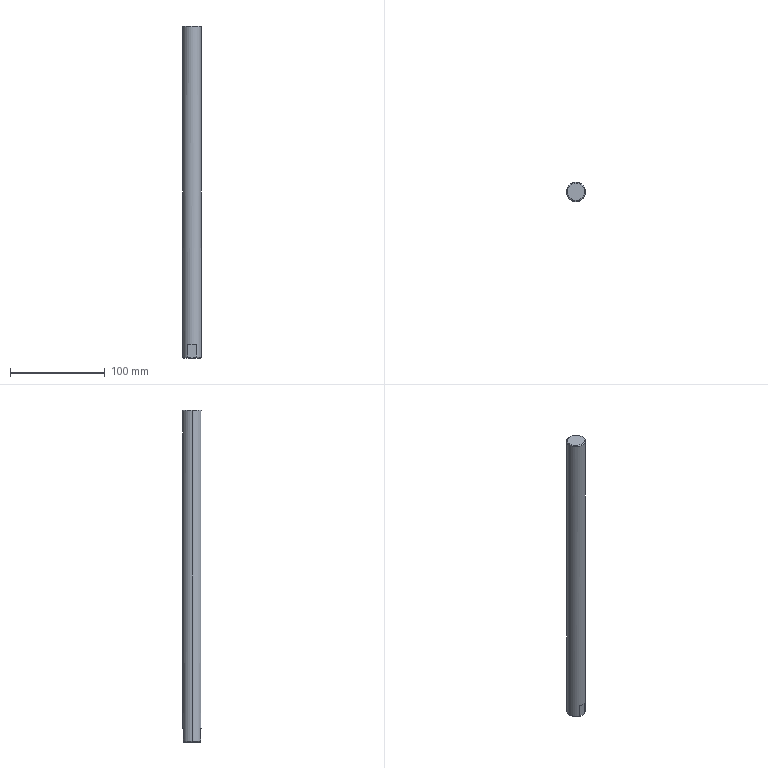Part | STEP file | KF-2212-050-003 | 1 solid | 17 faces | box 20 x 20 x 350 mm | volume 109026 mm3 | plane 6 | torus 5 | cylinder 4 | cone 2 | commonest cylinder face diameters 6.8 x2 20 x2
STEP:
#1=CARTESIAN_POINT('',(3.4,0.,19.75));
#2=VERTEX_POINT('',#1);
#3=CARTESIAN_POINT('',(-3.4,0.,19.75));
#4=VERTEX_POINT('',#3);
#5=CARTESIAN_POINT('',(0.,0.,19.75));
#6=DIRECTION('',(0.,0.,-1.));
#7=DIRECTION('',(-1.,0.,0.));
#8=AXIS2_PLACEMENT_3D('',#5,#6,#7);
#9=CIRCLE('',#8,3.4);
#10=EDGE_CURVE('',#2,#4,#9,.T.);
#11=ORIENTED_EDGE('',*,*,#10,.F.);
#12=CARTESIAN_POINT('',(3.4,0.,0.));
#13=VERTEX_POINT('',#12);
#14=CARTESIAN_POINT('',(3.4,0.,0.));
#15=DIRECTION('',(0.,0.,-1.));
#16=VECTOR('',#15,1000.);
#17=LINE('',#14,#16);
#18=EDGE_CURVE('',#2,#13,#17,.T.);
#19=ORIENTED_EDGE('',*,*,#18,.T.);
#20=CARTESIAN_POINT('',(-3.4,0.,0.));
#21=VERTEX_POINT('',#20);
#22=CARTESIAN_POINT('',(0.,0.,0.));
#23=DIRECTION('',(0.,0.,-1.));
#24=DIRECTION('',(-1.,0.,0.));
#25=AXIS2_PLACEMENT_3D('',#22,#23,#24);
#26=CIRCLE('',#25,3.4);
#27=EDGE_CURVE('',#13,#21,#26,.T.);
#28=ORIENTED_EDGE('',*,*,#27,.T.);
#29=CARTESIAN_POINT('',(-3.4,0.,0.));
#30=DIRECTION('',(0.,0.,-1.));
#31=VECTOR('',#30,1000.);
#32=LINE('',#29,#31);
#33=EDGE_CURVE('',#4,#21,#32,.T.);
#34=ORIENTED_EDGE('',*,*,#33,.F.);
#35=EDGE_LOOP('',(#11,#19,#28,#34));
#36=FACE_OUTER_BOUND('',#35,.T.);
#37=CARTESIAN_POINT('',(0.,0.,0.));
#38=DIRECTION('',(0.,0.,-1.));
#39=DIRECTION('',(-1.,0.,0.));
#40=AXIS2_PLACEMENT_3D('',#37,#38,#39);
#41=CYLINDRICAL_SURFACE('',#40,3.4);
#42=ADVANCED_FACE('',(#36),#41,.F.);
#43=CARTESIAN_POINT('',(0.,0.,21.793));
#44=VERTEX_POINT('',#43);
#45=CARTESIAN_POINT('',(-3.4,0.,19.75));
#46=DIRECTION('',(-0.8572,0.,-0.515));
#47=VECTOR('',#46,1000.);
#48=LINE('',#45,#47);
#49=EDGE_CURVE('',#44,#4,#48,.T.);
#50=ORIENTED_EDGE('',*,*,#49,.F.);
#51=CARTESIAN_POINT('',(3.4,0.,19.75));
#52=DIRECTION('',(0.8572,0.,-0.515));
#53=VECTOR('',#52,1000.);
#54=LINE('',#51,#53);
#55=EDGE_CURVE('',#44,#2,#54,.T.);
#56=ORIENTED_EDGE('',*,*,#55,.T.);
#57=ORIENTED_EDGE('',*,*,#10,.T.);
#58=EDGE_LOOP('',(#50,#56,#57));
#59=FACE_OUTER_BOUND('',#58,.T.);
#60=CARTESIAN_POINT('',(0.,0.,19.75));
#61=DIRECTION('',(0.,0.,-1.));
#62=DIRECTION('',(-1.,0.,0.));
#63=AXIS2_PLACEMENT_3D('',#60,#61,#62);
#64=CONICAL_SURFACE('',#63,3.4,1.03);
#65=ADVANCED_FACE('',(#59),#64,.F.);
#66=CARTESIAN_POINT('',(9.,0.,0.));
#67=VERTEX_POINT('',#66);
#68=CARTESIAN_POINT('',(0.,-9.,0.));
#69=VERTEX_POINT('',#68);
#70=CARTESIAN_POINT('',(0.,0.,0.));
#71=DIRECTION('',(0.,0.,-1.));
#72=DIRECTION('',(1.,0.,0.));
#73=AXIS2_PLACEMENT_3D('',#70,#71,#72);
#74=CIRCLE('',#73,9.);
#75=EDGE_CURVE('',#67,#69,#74,.T.);
#76=ORIENTED_EDGE('',*,*,#75,.F.);
#77=CARTESIAN_POINT('',(10.,0.,1.));
#78=VERTEX_POINT('',#77);
#79=CARTESIAN_POINT('',(9.,0.,1.));
#80=DIRECTION('',(0.,-1.,0.));
#81=DIRECTION('',(0.,0.,-1.));
#82=AXIS2_PLACEMENT_3D('',#79,#80,#81);
#83=CIRCLE('',#82,1.);
#84=EDGE_CURVE('',#67,#78,#83,.T.);
#85=ORIENTED_EDGE('',*,*,#84,.T.);
#86=CARTESIAN_POINT('',(4.359,-9.,1.));
#87=VERTEX_POINT('',#86);
#88=CARTESIAN_POINT('',(0.,0.,1.));
#89=DIRECTION('',(0.,0.,1.));
#90=DIRECTION('',(1.,0.,0.));
#91=AXIS2_PLACEMENT_3D('',#88,#89,#90);
#92=CIRCLE('',#91,10.);
#93=EDGE_CURVE('',#87,#78,#92,.T.);
#94=ORIENTED_EDGE('',*,*,#93,.F.);
#95=CARTESIAN_POINT('',(0.,-9.,0.));
#96=CARTESIAN_POINT('',(0.3943,-9.,0.));
#97=CARTESIAN_POINT('',(0.7886,-9.,-0.0009886));
#98=CARTESIAN_POINT('',(1.577,-9.,0.006989));
#99=CARTESIAN_POINT('',(1.972,-9.,0.01581));
#100=CARTESIAN_POINT('',(2.561,-9.,0.06379));
#101=CARTESIAN_POINT('',(2.756,-9.,0.0857));
#102=CARTESIAN_POINT('',(3.144,-9.,0.1503));
#103=CARTESIAN_POINT('',(3.339,-9.,0.1931));
#104=CARTESIAN_POINT('',(3.62,-9.,0.2846));
#105=CARTESIAN_POINT('',(3.712,-9.,0.3197));
#106=CARTESIAN_POINT('',(3.89,-9.,0.4033));
#107=CARTESIAN_POINT('',(3.977,-9.,0.4522));
#108=CARTESIAN_POINT('',(4.137,-9.,0.5697));
#109=CARTESIAN_POINT('',(4.211,-9.,0.6387));
#110=CARTESIAN_POINT('',(4.322,-9.,0.8026));
#111=CARTESIAN_POINT('',(4.359,-9.,0.9011));
#112=CARTESIAN_POINT('',(4.359,-9.,1.));
#113=B_SPLINE_CURVE_WITH_KNOTS('',3,(#95,#96,#97,#98,#99,#100,#101,#102,#103,#104,#105,#106,#107,#108,#109,#110,#111,#112),.UNSPECIFIED.,.F.,.F.,(4,2,2,2,2,2,2,2,4),(0.,0.001183,0.002366,0.002957,0.003549,0.003844,0.00414,0.004436,0.004731),.UNSPECIFIED.);
#114=EDGE_CURVE('',#69,#87,#113,.T.);
#115=ORIENTED_EDGE('',*,*,#114,.F.);
#116=EDGE_LOOP('',(#76,#85,#94,#115));
#117=FACE_OUTER_BOUND('',#116,.T.);
#118=CARTESIAN_POINT('',(0.,0.,1.));
#119=DIRECTION('',(0.,0.,1.));
#120=DIRECTION('',(1.,0.,0.));
#121=AXIS2_PLACEMENT_3D('',#118,#119,#120);
#122=TOROIDAL_SURFACE('',#121,9.,1.);
#123=ADVANCED_FACE('',(#117),#122,.T.);
#124=CARTESIAN_POINT('',(-10.,0.,349.));
#125=VERTEX_POINT('',#124);
#126=CARTESIAN_POINT('',(10.,0.,349.));
#127=VERTEX_POINT('',#126);
#128=CARTESIAN_POINT('',(0.,0.,349.));
#129=DIRECTION('',(0.,0.,-1.));
#130=DIRECTION('',(1.,0.,0.));
#131=AXIS2_PLACEMENT_3D('',#128,#129,#130);
#132=CIRCLE('',#131,10.);
#133=EDGE_CURVE('',#125,#127,#132,.T.);
#134=ORIENTED_EDGE('',*,*,#133,.F.);
#135=CARTESIAN_POINT('',(-9.,0.,350.));
#136=VERTEX_POINT('',#135);
#137=CARTESIAN_POINT('',(-9.,0.,349.));
#138=DIRECTION('',(0.,1.,0.));
#139=DIRECTION('',(-1.,0.,0.));
#140=AXIS2_PLACEMENT_3D('',#137,#138,#139);
#141=CIRCLE('',#140,1.);
#142=EDGE_CURVE('',#125,#136,#141,.T.);
#143=ORIENTED_EDGE('',*,*,#142,.T.);
#144=CARTESIAN_POINT('',(9.,0.,350.));
#145=VERTEX_POINT('',#144);
#146=CARTESIAN_POINT('',(0.,0.,350.));
#147=DIRECTION('',(0.,0.,1.));
#148=DIRECTION('',(1.,0.,0.));
#149=AXIS2_PLACEMENT_3D('',#146,#147,#148);
#150=CIRCLE('',#149,9.);
#151=EDGE_CURVE('',#145,#136,#150,.T.);
#152=ORIENTED_EDGE('',*,*,#151,.F.);
#153=CARTESIAN_POINT('',(9.,0.,349.));
#154=DIRECTION('',(0.,-1.,0.));
#155=DIRECTION('',(0.,0.,-1.));
#156=AXIS2_PLACEMENT_3D('',#153,#154,#155);
#157=CIRCLE('',#156,1.);
#158=EDGE_CURVE('',#127,#145,#157,.T.);
#159=ORIENTED_EDGE('',*,*,#158,.F.);
#160=EDGE_LOOP('',(#134,#143,#152,#159));
#161=FACE_OUTER_BOUND('',#160,.T.);
#162=CARTESIAN_POINT('',(0.,0.,349.));
#163=DIRECTION('',(0.,0.,1.));
#164=DIRECTION('',(1.,0.,0.));
#165=AXIS2_PLACEMENT_3D('',#162,#163,#164);
#166=TOROIDAL_SURFACE('',#165,9.,1.);
#167=ADVANCED_FACE('',(#161),#166,.T.);
#168=ORIENTED_EDGE('',*,*,#133,.T.);
#169=CARTESIAN_POINT('',(10.,0.,350.));
#170=DIRECTION('',(0.,0.,-1.));
#171=VECTOR('',#170,1000.);
#172=LINE('',#169,#171);
#173=EDGE_CURVE('',#127,#78,#172,.T.);
#174=ORIENTED_EDGE('',*,*,#173,.T.);
#175=CARTESIAN_POINT('',(4.359,9.,1.));
#176=VERTEX_POINT('',#175);
#177=CARTESIAN_POINT('',(0.,0.,1.));
#178=DIRECTION('',(0.,0.,1.));
#179=DIRECTION('',(1.,0.,0.));
#180=AXIS2_PLACEMENT_3D('',#177,#178,#179);
#181=CIRCLE('',#180,10.);
#182=EDGE_CURVE('',#78,#176,#181,.T.);
#183=ORIENTED_EDGE('',*,*,#182,.T.);
#184=CARTESIAN_POINT('',(4.359,9.,14.));
#185=VERTEX_POINT('',#184);
#186=CARTESIAN_POINT('',(4.359,9.,350.));
#187=DIRECTION('',(0.,0.,1.));
#188=VECTOR('',#187,1000.);
#189=LINE('',#186,#188);
#190=EDGE_CURVE('',#176,#185,#189,.T.);
#191=ORIENTED_EDGE('',*,*,#190,.T.);
#192=CARTESIAN_POINT('',(-4.359,9.,14.));
#193=VERTEX_POINT('',#192);
#194=CARTESIAN_POINT('',(0.,0.,14.));
#195=DIRECTION('',(0.,0.,-1.));
#196=DIRECTION('',(-1.,0.,0.));
#197=AXIS2_PLACEMENT_3D('',#194,#195,#196);
#198=CIRCLE('',#197,10.);
#199=EDGE_CURVE('',#193,#185,#198,.T.);
#200=ORIENTED_EDGE('',*,*,#199,.F.);
#201=CARTESIAN_POINT('',(-4.359,9.,1.));
#202=VERTEX_POINT('',#201);
#203=CARTESIAN_POINT('',(-4.359,9.,350.));
#204=DIRECTION('',(0.,0.,-1.));
#205=VECTOR('',#204,1000.);
#206=LINE('',#203,#205);
#207=EDGE_CURVE('',#193,#202,#206,.T.);
#208=ORIENTED_EDGE('',*,*,#207,.T.);
#209=CARTESIAN_POINT('',(-10.,0.,1.));
#210=VERTEX_POINT('',#209);
#211=CARTESIAN_POINT('',(0.,0.,1.));
#212=DIRECTION('',(0.,0.,1.));
#213=DIRECTION('',(1.,0.,0.));
#214=AXIS2_PLACEMENT_3D('',#211,#212,#213);
#215=CIRCLE('',#214,10.);
#216=EDGE_CURVE('',#202,#210,#215,.T.);
#217=ORIENTED_EDGE('',*,*,#216,.T.);
#218=CARTESIAN_POINT('',(-10.,0.,350.));
#219=DIRECTION('',(0.,0.,-1.));
#220=VECTOR('',#219,1000.);
#221=LINE('',#218,#220);
#222=EDGE_CURVE('',#125,#210,#221,.T.);
#223=ORIENTED_EDGE('',*,*,#222,.F.);
#224=EDGE_LOOP('',(#168,#174,#183,#191,#200,#208,#217,#223));
#225=FACE_OUTER_BOUND('',#224,.T.);
#226=CARTESIAN_POINT('',(0.,0.,350.));
#227=DIRECTION('',(0.,0.,-1.));
#228=DIRECTION('',(-1.,0.,0.));
#229=AXIS2_PLACEMENT_3D('',#226,#227,#228);
#230=CYLINDRICAL_SURFACE('',#229,10.);
#231=ADVANCED_FACE('',(#225),#230,.T.);
#232=CARTESIAN_POINT('',(0.,9.,0.));
#233=VERTEX_POINT('',#232);
#234=CARTESIAN_POINT('',(0.,9.,0.));
#235=CARTESIAN_POINT('',(-0.3943,9.,0.));
#236=CARTESIAN_POINT('',(-0.7886,9.,-0.0009886));
#237=CARTESIAN_POINT('',(-1.577,9.,0.006989));
#238=CARTESIAN_POINT('',(-1.972,9.,0.01581));
#239=CARTESIAN_POINT('',(-2.561,9.,0.06379));
#240=CARTESIAN_POINT('',(-2.756,9.,0.0857));
#241=CARTESIAN_POINT('',(-3.144,9.,0.1503));
#242=CARTESIAN_POINT('',(-3.339,9.,0.1931));
#243=CARTESIAN_POINT('',(-3.62,9.,0.2846));
#244=CARTESIAN_POINT('',(-3.712,9.,0.3197));
#245=CARTESIAN_POINT('',(-3.89,9.,0.4033));
#246=CARTESIAN_POINT('',(-3.977,9.,0.4522));
#247=CARTESIAN_POINT('',(-4.137,9.,0.5697));
#248=CARTESIAN_POINT('',(-4.211,9.,0.6387));
#249=CARTESIAN_POINT('',(-4.322,9.,0.8026));
#250=CARTESIAN_POINT('',(-4.359,9.,0.9011));
#251=CARTESIAN_POINT('',(-4.359,9.,1.));
#252=B_SPLINE_CURVE_WITH_KNOTS('',3,(#234,#235,#236,#237,#238,#239,#240,#241,#242,#243,#244,#245,#246,#247,#248,#249,#250,#251),.UNSPECIFIED.,.F.,.F.,(4,2,2,2,2,2,2,2,4),(0.,0.001183,0.002366,0.002957,0.003549,0.003844,0.00414,0.004436,0.004731),.UNSPECIFIED.);
#253=EDGE_CURVE('',#233,#202,#252,.T.);
#254=ORIENTED_EDGE('',*,*,#253,.F.);
#255=CARTESIAN_POINT('',(0.,0.,0.));
#256=DIRECTION('',(0.,0.,-1.));
#257=DIRECTION('',(1.,0.,0.));
#258=AXIS2_PLACEMENT_3D('',#255,#256,#257);
#259=CIRCLE('',#258,9.);
#260=EDGE_CURVE('',#69,#233,#259,.T.);
#261=ORIENTED_EDGE('',*,*,#260,.F.);
#262=CARTESIAN_POINT('',(-4.359,-9.,1.));
#263=VERTEX_POINT('',#262);
#264=CARTESIAN_POINT('',(-4.359,-9.,1.));
#265=CARTESIAN_POINT('',(-4.359,-9.,0.901));
#266=CARTESIAN_POINT('',(-4.322,-9.,0.802));
#267=CARTESIAN_POINT('',(-4.21,-9.,0.6373));
#268=CARTESIAN_POINT('',(-4.136,-9.,0.5681));
#269=CARTESIAN_POINT('',(-3.895,-9.,0.3927));
#270=CARTESIAN_POINT('',(-3.709,-9.,0.3135));
#271=CARTESIAN_POINT('',(-3.335,-9.,0.1923));
#272=CARTESIAN_POINT('',(-3.143,-9.,0.1501));
#273=CARTESIAN_POINT('',(-2.754,-9.,0.08543));
#274=CARTESIAN_POINT('',(-2.557,-9.,0.06343));
#275=CARTESIAN_POINT('',(-1.968,-9.,0.01564));
#276=CARTESIAN_POINT('',(-1.575,-9.,0.006949));
#277=CARTESIAN_POINT('',(-0.9844,-9.,0.001));
#278=CARTESIAN_POINT('',(-0.7875,-9.,0.0004371));
#279=CARTESIAN_POINT('',(-0.3938,-9.,-0.00006223));
#280=CARTESIAN_POINT('',(-0.1985,-9.,0.));
#281=CARTESIAN_POINT('',(0.,-9.,0.));
#282=B_SPLINE_CURVE_WITH_KNOTS('',3,(#264,#265,#266,#267,#268,#269,#270,#271,#272,#273,#274,#275,#276,#277,#278,#279,#280,#281),.UNSPECIFIED.,.F.,.F.,(4,2,2,2,2,2,2,2,4),(0.01425,0.01455,0.01485,0.01545,0.01604,0.01664,0.01783,0.01842,0.01902),.UNSPECIFIED.);
#283=EDGE_CURVE('',#263,#69,#282,.T.);
#284=ORIENTED_EDGE('',*,*,#283,.F.);
#285=CARTESIAN_POINT('',(0.,0.,1.));
#286=DIRECTION('',(0.,0.,1.));
#287=DIRECTION('',(1.,0.,0.));
#288=AXIS2_PLACEMENT_3D('',#285,#286,#287);
#289=CIRCLE('',#288,10.);
#290=EDGE_CURVE('',#210,#263,#289,.T.);
#291=ORIENTED_EDGE('',*,*,#290,.F.);
#292=ORIENTED_EDGE('',*,*,#216,.F.);
#293=EDGE_LOOP('',(#254,#261,#284,#291,#292));
#294=FACE_OUTER_BOUND('',#293,.T.);
#295=CARTESIAN_POINT('',(0.,0.,1.));
#296=DIRECTION('',(0.,0.,1.));
#297=DIRECTION('',(1.,0.,0.));
#298=AXIS2_PLACEMENT_3D('',#295,#296,#297);
#299=TOROIDAL_SURFACE('',#298,9.,1.);
#300=ADVANCED_FACE('',(#294),#299,.T.);
#301=ORIENTED_EDGE('',*,*,#173,.F.);
#302=CARTESIAN_POINT('',(0.,0.,349.));
#303=DIRECTION('',(0.,0.,-1.));
#304=DIRECTION('',(1.,0.,0.));
#305=AXIS2_PLACEMENT_3D('',#302,#303,#304);
#306=CIRCLE('',#305,10.);
#307=EDGE_CURVE('',#127,#125,#306,.T.);
#308=ORIENTED_EDGE('',*,*,#307,.T.);
#309=ORIENTED_EDGE('',*,*,#222,.T.);
#310=ORIENTED_EDGE('',*,*,#290,.T.);
#311=CARTESIAN_POINT('',(-4.359,-9.,14.));
#312=VERTEX_POINT('',#311);
#313=CARTESIAN_POINT('',(-4.359,-9.,350.));
#314=DIRECTION('',(0.,0.,1.));
#315=VECTOR('',#314,1000.);
#316=LINE('',#313,#315);
#317=EDGE_CURVE('',#263,#312,#316,.T.);
#318=ORIENTED_EDGE('',*,*,#317,.T.);
#319=CARTESIAN_POINT('',(4.359,-9.,14.));
#320=VERTEX_POINT('',#319);
#321=CARTESIAN_POINT('',(0.,0.,14.));
#322=DIRECTION('',(0.,0.,1.));
#323=DIRECTION('',(1.,0.,0.));
#324=AXIS2_PLACEMENT_3D('',#321,#322,#323);
#325=CIRCLE('',#324,10.);
#326=EDGE_CURVE('',#312,#320,#325,.T.);
#327=ORIENTED_EDGE('',*,*,#326,.T.);
#328=CARTESIAN_POINT('',(4.359,-9.,350.));
#329=DIRECTION('',(0.,0.,-1.));
#330=VECTOR('',#329,1000.);
#331=LINE('',#328,#330);
#332=EDGE_CURVE('',#320,#87,#331,.T.);
#333=ORIENTED_EDGE('',*,*,#332,.T.);
#334=ORIENTED_EDGE('',*,*,#93,.T.);
#335=EDGE_LOOP('',(#301,#308,#309,#310,#318,#327,#333,#334));
#336=FACE_OUTER_BOUND('',#335,.T.);
#337=CARTESIAN_POINT('',(0.,0.,350.));
#338=DIRECTION('',(0.,0.,-1.));
#339=DIRECTION('',(-1.,0.,0.));
#340=AXIS2_PLACEMENT_3D('',#337,#338,#339);
#341=CYLINDRICAL_SURFACE('',#340,10.);
#342=ADVANCED_FACE('',(#336),#341,.T.);
#343=ORIENTED_EDGE('',*,*,#151,.T.);
#344=CARTESIAN_POINT('',(0.,0.,350.));
#345=DIRECTION('',(0.,0.,1.));
#346=DIRECTION('',(1.,0.,0.));
#347=AXIS2_PLACEMENT_3D('',#344,#345,#346);
#348=CIRCLE('',#347,9.);
#349=EDGE_CURVE('',#136,#145,#348,.T.);
#350=ORIENTED_EDGE('',*,*,#349,.T.);
#351=EDGE_LOOP('',(#343,#350));
#352=FACE_OUTER_BOUND('',#351,.T.);
#353=CARTESIAN_POINT('',(0.,0.,350.));
#354=DIRECTION('',(0.,0.,1.));
#355=DIRECTION('',(1.,0.,0.));
#356=AXIS2_PLACEMENT_3D('',#353,#354,#355);
#357=PLANE('',#356);
#358=ADVANCED_FACE('',(#352),#357,.T.);
#359=CARTESIAN_POINT('',(0.,0.,0.));
#360=DIRECTION('',(0.,0.,-1.));
#361=DIRECTION('',(-1.,0.,0.));
#362=AXIS2_PLACEMENT_3D('',#359,#360,#361);
#363=CIRCLE('',#362,3.4);
#364=EDGE_CURVE('',#21,#13,#363,.T.);
#365=ORIENTED_EDGE('',*,*,#364,.F.);
#366=ORIENTED_EDGE('',*,*,#27,.F.);
#367=EDGE_LOOP('',(#365,#366));
#368=FACE_BOUND('',#367,.T.);
#369=ORIENTED_EDGE('',*,*,#260,.T.);
#370=CARTESIAN_POINT('',(0.,0.,0.));
#371=DIRECTION('',(0.,0.,-1.));
#372=DIRECTION('',(1.,0.,0.));
#373=AXIS2_PLACEMENT_3D('',#370,#371,#372);
#374=CIRCLE('',#373,9.);
#375=EDGE_CURVE('',#233,#67,#374,.T.);
#376=ORIENTED_EDGE('',*,*,#375,.T.);
#377=ORIENTED_EDGE('',*,*,#75,.T.);
#378=EDGE_LOOP('',(#369,#376,#377));
#379=FACE_OUTER_BOUND('',#378,.T.);
#380=CARTESIAN_POINT('',(0.,0.,0.));
#381=DIRECTION('',(0.,0.,1.));
#382=DIRECTION('',(1.,0.,0.));
#383=AXIS2_PLACEMENT_3D('',#380,#381,#382);
#384=PLANE('',#383);
#385=ADVANCED_FACE('',(#368,#379),#384,.F.);
#386=ORIENTED_EDGE('',*,*,#142,.F.);
#387=ORIENTED_EDGE('',*,*,#307,.F.);
#388=ORIENTED_EDGE('',*,*,#158,.T.);
#389=ORIENTED_EDGE('',*,*,#349,.F.);
#390=EDGE_LOOP('',(#386,#387,#388,#389));
#391=FACE_OUTER_BOUND('',#390,.T.);
#392=CARTESIAN_POINT('',(0.,0.,349.));
#393=DIRECTION('',(0.,0.,1.));
#394=DIRECTION('',(1.,0.,0.));
#395=AXIS2_PLACEMENT_3D('',#392,#393,#394);
#396=TOROIDAL_SURFACE('',#395,9.,1.);
#397=ADVANCED_FACE('',(#391),#396,.T.);
#398=ORIENTED_EDGE('',*,*,#84,.F.);
#399=ORIENTED_EDGE('',*,*,#375,.F.);
#400=CARTESIAN_POINT('',(4.359,9.,1.));
#401=CARTESIAN_POINT('',(4.359,9.,0.901));
#402=CARTESIAN_POINT('',(4.322,9.,0.802));
#403=CARTESIAN_POINT('',(4.21,9.,0.6373));
#404=CARTESIAN_POINT('',(4.136,9.,0.5681));
#405=CARTESIAN_POINT('',(3.895,9.,0.3927));
#406=CARTESIAN_POINT('',(3.709,9.,0.3135));
#407=CARTESIAN_POINT('',(3.335,9.,0.1923));
#408=CARTESIAN_POINT('',(3.143,9.,0.1501));
#409=CARTESIAN_POINT('',(2.754,9.,0.08543));
#410=CARTESIAN_POINT('',(2.557,9.,0.06343));
#411=CARTESIAN_POINT('',(1.968,9.,0.01564));
#412=CARTESIAN_POINT('',(1.575,9.,0.006949));
#413=CARTESIAN_POINT('',(0.9844,9.,0.001));
#414=CARTESIAN_POINT('',(0.7875,9.,0.0004371));
#415=CARTESIAN_POINT('',(0.3938,9.,-0.00006223));
#416=CARTESIAN_POINT('',(0.1985,9.,0.));
#417=CARTESIAN_POINT('',(0.,9.,0.));
#418=B_SPLINE_CURVE_WITH_KNOTS('',3,(#400,#401,#402,#403,#404,#405,#406,#407,#408,#409,#410,#411,#412,#413,#414,#415,#416,#417),.UNSPECIFIED.,.F.,.F.,(4,2,2,2,2,2,2,2,4),(0.01425,0.01455,0.01485,0.01545,0.01604,0.01664,0.01783,0.01842,0.01902),.UNSPECIFIED.);
#419=EDGE_CURVE('',#176,#233,#418,.T.);
#420=ORIENTED_EDGE('',*,*,#419,.F.);
#421=ORIENTED_EDGE('',*,*,#182,.F.);
#422=EDGE_LOOP('',(#398,#399,#420,#421));
#423=FACE_OUTER_BOUND('',#422,.T.);
#424=CARTESIAN_POINT('',(0.,0.,1.));
#425=DIRECTION('',(0.,0.,1.));
#426=DIRECTION('',(1.,0.,0.));
#427=AXIS2_PLACEMENT_3D('',#424,#425,#426);
#428=TOROIDAL_SURFACE('',#427,9.,1.);
#429=ADVANCED_FACE('',(#423),#428,.T.);
#430=ORIENTED_EDGE('',*,*,#55,.F.);
#431=ORIENTED_EDGE('',*,*,#49,.T.);
#432=CARTESIAN_POINT('',(0.,0.,19.75));
#433=DIRECTION('',(0.,0.,-1.));
#434=DIRECTION('',(-1.,0.,0.));
#435=AXIS2_PLACEMENT_3D('',#432,#433,#434);
#436=CIRCLE('',#435,3.4);
#437=EDGE_CURVE('',#4,#2,#436,.T.);
#438=ORIENTED_EDGE('',*,*,#437,.T.);
#439=EDGE_LOOP('',(#430,#431,#438));
#440=FACE_OUTER_BOUND('',#439,.T.);
#441=CARTESIAN_POINT('',(0.,0.,19.75));
#442=DIRECTION('',(0.,0.,-1.));
#443=DIRECTION('',(-1.,0.,0.));
#444=AXIS2_PLACEMENT_3D('',#441,#442,#443);
#445=CONICAL_SURFACE('',#444,3.4,1.03);
#446=ADVANCED_FACE('',(#440),#445,.F.);
#447=ORIENTED_EDGE('',*,*,#18,.F.);
#448=ORIENTED_EDGE('',*,*,#437,.F.);
#449=ORIENTED_EDGE('',*,*,#33,.T.);
#450=ORIENTED_EDGE('',*,*,#364,.T.);
#451=EDGE_LOOP('',(#447,#448,#449,#450));
#452=FACE_OUTER_BOUND('',#451,.T.);
#453=CARTESIAN_POINT('',(0.,0.,0.));
#454=DIRECTION('',(0.,0.,-1.));
#455=DIRECTION('',(-1.,0.,0.));
#456=AXIS2_PLACEMENT_3D('',#453,#454,#455);
#457=CYLINDRICAL_SURFACE('',#456,3.4);
#458=ADVANCED_FACE('',(#452),#457,.F.);
#459=CARTESIAN_POINT('',(10.871,-9.,14.));
#460=DIRECTION('',(1.,0.,0.));
#461=VECTOR('',#460,1000.);
#462=LINE('',#459,#461);
#463=EDGE_CURVE('',#312,#320,#462,.T.);
#464=ORIENTED_EDGE('',*,*,#463,.T.);
#465=ORIENTED_EDGE('',*,*,#326,.F.);
#466=EDGE_LOOP('',(#464,#465));
#467=FACE_OUTER_BOUND('',#466,.T.);
#468=CARTESIAN_POINT('',(0.,0.,14.));
#469=DIRECTION('',(0.,0.,1.));
#470=DIRECTION('',(1.,0.,0.));
#471=AXIS2_PLACEMENT_3D('',#468,#469,#470);
#472=PLANE('',#471);
#473=ADVANCED_FACE('',(#467),#472,.F.);
#474=ORIENTED_EDGE('',*,*,#463,.F.);
#475=ORIENTED_EDGE('',*,*,#317,.F.);
#476=ORIENTED_EDGE('',*,*,#283,.T.);
#477=ORIENTED_EDGE('',*,*,#114,.T.);
#478=ORIENTED_EDGE('',*,*,#332,.F.);
#479=EDGE_LOOP('',(#474,#475,#476,#477,#478));
#480=FACE_OUTER_BOUND('',#479,.T.);
#481=CARTESIAN_POINT('',(10.871,-9.,14.));
#482=DIRECTION('',(0.,1.,0.));
#483=DIRECTION('',(-1.,0.,0.));
#484=AXIS2_PLACEMENT_3D('',#481,#482,#483);
#485=PLANE('',#484);
#486=ADVANCED_FACE('',(#480),#485,.F.);
#487=ORIENTED_EDGE('',*,*,#199,.T.);
#488=CARTESIAN_POINT('',(14.799,9.,14.));
#489=DIRECTION('',(-1.,0.,0.));
#490=VECTOR('',#489,1000.);
#491=LINE('',#488,#490);
#492=EDGE_CURVE('',#185,#193,#491,.T.);
#493=ORIENTED_EDGE('',*,*,#492,.T.);
#494=EDGE_LOOP('',(#487,#493));
#495=FACE_OUTER_BOUND('',#494,.T.);
#496=CARTESIAN_POINT('',(0.,0.,14.));
#497=DIRECTION('',(0.,0.,-1.));
#498=DIRECTION('',(-1.,0.,0.));
#499=AXIS2_PLACEMENT_3D('',#496,#497,#498);
#500=PLANE('',#499);
#501=ADVANCED_FACE('',(#495),#500,.T.);
#502=ORIENTED_EDGE('',*,*,#492,.F.);
#503=ORIENTED_EDGE('',*,*,#190,.F.);
#504=ORIENTED_EDGE('',*,*,#419,.T.);
#505=ORIENTED_EDGE('',*,*,#253,.T.);
#506=ORIENTED_EDGE('',*,*,#207,.F.);
#507=EDGE_LOOP('',(#502,#503,#504,#505,#506));
#508=FACE_OUTER_BOUND('',#507,.T.);
#509=CARTESIAN_POINT('',(14.799,9.,14.));
#510=DIRECTION('',(0.,-1.,0.));
#511=DIRECTION('',(0.,0.,-1.));
#512=AXIS2_PLACEMENT_3D('',#509,#510,#511);
#513=PLANE('',#512);
#514=ADVANCED_FACE('',(#508),#513,.F.);
#515=CLOSED_SHELL('',(#42,#65,#123,#167,#231,#300,#342,#358,#385,#397,#429,#446,#458,#473,#486,#501,#514));
#516=MANIFOLD_SOLID_BREP('',#515);
#517=CARTESIAN_POINT('',(0.,0.,0.));
#518=DIRECTION('',(0.,0.,1.));
#519=DIRECTION('',(1.,0.,0.));
#520=AXIS2_PLACEMENT_3D('',#517,#518,#519);
#521=(LENGTH_UNIT()NAMED_UNIT(*)SI_UNIT(.MILLI.,.METRE.));
#522=UNCERTAINTY_MEASURE_WITH_UNIT(LENGTH_MEASURE(0.00001),#521,'','');
#523=(NAMED_UNIT(*)PLANE_ANGLE_UNIT()SI_UNIT($,.RADIAN.));
#524=(NAMED_UNIT(*)SI_UNIT($,.STERADIAN.)SOLID_ANGLE_UNIT());
#525=(GEOMETRIC_REPRESENTATION_CONTEXT(3)GLOBAL_UNCERTAINTY_ASSIGNED_CONTEXT((#522))GLOBAL_UNIT_ASSIGNED_CONTEXT((#521,#523,#524))REPRESENTATION_CONTEXT('',''));
#526=ADVANCED_BREP_SHAPE_REPRESENTATION('',(#516,#520),#525);